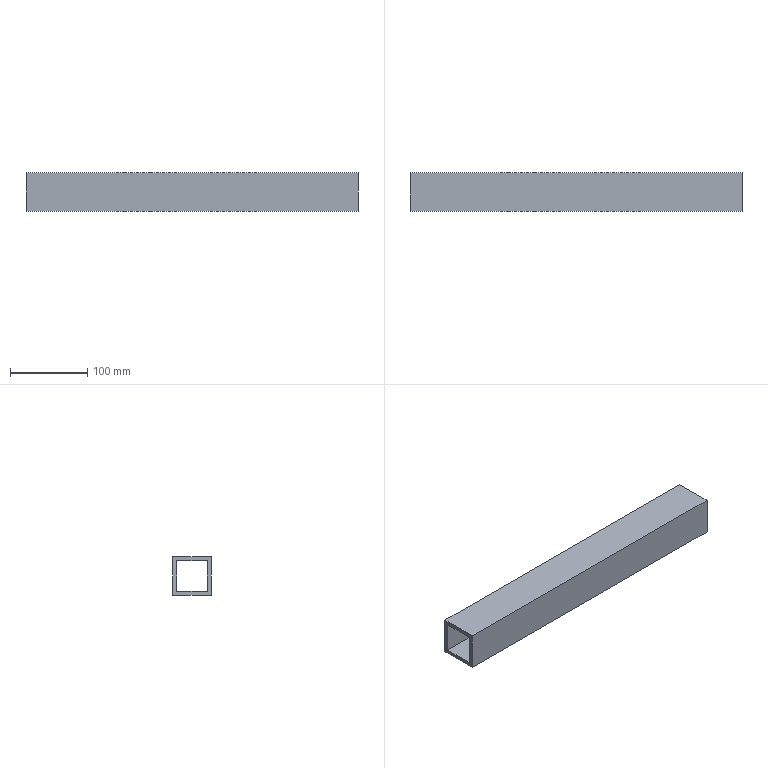Part | NX | features solid 2 | 1 solid | 10 faces | box 430 x 50 x 50 mm | volume 387000 mm3 | plane 10
STEP:
#1=CARTESIAN_POINT('',(630.,520.,-560.));
#2=VERTEX_POINT('',#1);
#3=CARTESIAN_POINT('',(630.,480.,-560.));
#4=VERTEX_POINT('',#3);
#5=CARTESIAN_POINT('',(630.,475.,-560.));
#6=DIRECTION('',(0.,-1.,0.));
#7=VECTOR('',#6,1000.);
#8=LINE('',#5,#7);
#9=EDGE_CURVE('',#2,#4,#8,.T.);
#10=ORIENTED_EDGE('',*,*,#9,.F.);
#11=CARTESIAN_POINT('',(630.,520.,-520.));
#12=VERTEX_POINT('',#11);
#13=CARTESIAN_POINT('',(630.,520.,-565.));
#14=DIRECTION('',(0.,0.,-1.));
#15=VECTOR('',#14,1000.);
#16=LINE('',#13,#15);
#17=EDGE_CURVE('',#12,#2,#16,.T.);
#18=ORIENTED_EDGE('',*,*,#17,.F.);
#19=CARTESIAN_POINT('',(630.,480.,-520.));
#20=VERTEX_POINT('',#19);
#21=CARTESIAN_POINT('',(630.,475.,-520.));
#22=DIRECTION('',(0.,1.,0.));
#23=VECTOR('',#22,1000.);
#24=LINE('',#21,#23);
#25=EDGE_CURVE('',#20,#12,#24,.T.);
#26=ORIENTED_EDGE('',*,*,#25,.F.);
#27=CARTESIAN_POINT('',(630.,480.,-565.));
#28=DIRECTION('',(0.,0.,1.));
#29=VECTOR('',#28,1000.);
#30=LINE('',#27,#29);
#31=EDGE_CURVE('',#4,#20,#30,.T.);
#32=ORIENTED_EDGE('',*,*,#31,.F.);
#33=EDGE_LOOP('',(#10,#18,#26,#32));
#34=FACE_BOUND('',#33,.T.);
#35=CARTESIAN_POINT('',(630.,475.,-515.));
#36=VERTEX_POINT('',#35);
#37=CARTESIAN_POINT('',(630.,525.,-515.));
#38=VERTEX_POINT('',#37);
#39=CARTESIAN_POINT('',(630.,475.,-515.));
#40=DIRECTION('',(0.,1.,0.));
#41=VECTOR('',#40,1000.);
#42=LINE('',#39,#41);
#43=EDGE_CURVE('',#36,#38,#42,.T.);
#44=ORIENTED_EDGE('',*,*,#43,.T.);
#45=CARTESIAN_POINT('',(630.,525.,-565.));
#46=VERTEX_POINT('',#45);
#47=CARTESIAN_POINT('',(630.,525.,-565.));
#48=DIRECTION('',(0.,0.,-1.));
#49=VECTOR('',#48,1000.);
#50=LINE('',#47,#49);
#51=EDGE_CURVE('',#38,#46,#50,.T.);
#52=ORIENTED_EDGE('',*,*,#51,.T.);
#53=CARTESIAN_POINT('',(630.,475.,-565.));
#54=VERTEX_POINT('',#53);
#55=CARTESIAN_POINT('',(630.,475.,-565.));
#56=DIRECTION('',(0.,-1.,0.));
#57=VECTOR('',#56,1000.);
#58=LINE('',#55,#57);
#59=EDGE_CURVE('',#46,#54,#58,.T.);
#60=ORIENTED_EDGE('',*,*,#59,.T.);
#61=CARTESIAN_POINT('',(630.,475.,-565.));
#62=DIRECTION('',(0.,0.,1.));
#63=VECTOR('',#62,1000.);
#64=LINE('',#61,#63);
#65=EDGE_CURVE('',#54,#36,#64,.T.);
#66=ORIENTED_EDGE('',*,*,#65,.T.);
#67=EDGE_LOOP('',(#44,#52,#60,#66));
#68=FACE_BOUND('',#67,.T.);
#69=CARTESIAN_POINT('',(630.,475.,-565.));
#70=DIRECTION('',(1.,0.,0.));
#71=DIRECTION('',(0.,-1.,0.));
#72=AXIS2_PLACEMENT_3D('',#69,#70,#71);
#73=PLANE('',#72);
#74=ADVANCED_FACE('',(#34,#68),#73,.F.);
#75=CARTESIAN_POINT('',(1060.,475.,-565.));
#76=VERTEX_POINT('',#75);
#77=CARTESIAN_POINT('',(640.,475.,-565.));
#78=DIRECTION('',(1.,0.,0.));
#79=VECTOR('',#78,1000.);
#80=LINE('',#77,#79);
#81=EDGE_CURVE('',#54,#76,#80,.T.);
#82=ORIENTED_EDGE('',*,*,#81,.T.);
#83=CARTESIAN_POINT('',(1060.,475.,-515.));
#84=VERTEX_POINT('',#83);
#85=CARTESIAN_POINT('',(1060.,475.,-565.));
#86=DIRECTION('',(0.,0.,-1.));
#87=VECTOR('',#86,1000.);
#88=LINE('',#85,#87);
#89=EDGE_CURVE('',#84,#76,#88,.T.);
#90=ORIENTED_EDGE('',*,*,#89,.F.);
#91=CARTESIAN_POINT('',(640.,475.,-515.));
#92=DIRECTION('',(-1.,0.,0.));
#93=VECTOR('',#92,1000.);
#94=LINE('',#91,#93);
#95=EDGE_CURVE('',#84,#36,#94,.T.);
#96=ORIENTED_EDGE('',*,*,#95,.T.);
#97=ORIENTED_EDGE('',*,*,#65,.F.);
#98=EDGE_LOOP('',(#82,#90,#96,#97));
#99=FACE_BOUND('',#98,.T.);
#100=CARTESIAN_POINT('',(640.,475.,-565.));
#101=DIRECTION('',(0.,1.,0.));
#102=DIRECTION('',(1.,0.,0.));
#103=AXIS2_PLACEMENT_3D('',#100,#101,#102);
#104=PLANE('',#103);
#105=ADVANCED_FACE('',(#99),#104,.F.);
#106=CARTESIAN_POINT('',(1060.,525.,-565.));
#107=VERTEX_POINT('',#106);
#108=CARTESIAN_POINT('',(640.,525.,-565.));
#109=DIRECTION('',(1.,0.,0.));
#110=VECTOR('',#109,1000.);
#111=LINE('',#108,#110);
#112=EDGE_CURVE('',#46,#107,#111,.T.);
#113=ORIENTED_EDGE('',*,*,#112,.T.);
#114=CARTESIAN_POINT('',(1060.,475.,-565.));
#115=DIRECTION('',(0.,1.,0.));
#116=VECTOR('',#115,1000.);
#117=LINE('',#114,#116);
#118=EDGE_CURVE('',#76,#107,#117,.T.);
#119=ORIENTED_EDGE('',*,*,#118,.F.);
#120=ORIENTED_EDGE('',*,*,#81,.F.);
#121=ORIENTED_EDGE('',*,*,#59,.F.);
#122=EDGE_LOOP('',(#113,#119,#120,#121));
#123=FACE_BOUND('',#122,.T.);
#124=CARTESIAN_POINT('',(640.,475.,-565.));
#125=DIRECTION('',(0.,0.,1.));
#126=DIRECTION('',(0.,-1.,0.));
#127=AXIS2_PLACEMENT_3D('',#124,#125,#126);
#128=PLANE('',#127);
#129=ADVANCED_FACE('',(#123),#128,.F.);
#130=CARTESIAN_POINT('',(1060.,525.,-515.));
#131=VERTEX_POINT('',#130);
#132=CARTESIAN_POINT('',(640.,525.,-515.));
#133=DIRECTION('',(1.,0.,0.));
#134=VECTOR('',#133,1000.);
#135=LINE('',#132,#134);
#136=EDGE_CURVE('',#38,#131,#135,.T.);
#137=ORIENTED_EDGE('',*,*,#136,.T.);
#138=CARTESIAN_POINT('',(1060.,525.,-515.));
#139=DIRECTION('',(0.,0.,1.));
#140=VECTOR('',#139,1000.);
#141=LINE('',#138,#140);
#142=EDGE_CURVE('',#107,#131,#141,.T.);
#143=ORIENTED_EDGE('',*,*,#142,.F.);
#144=ORIENTED_EDGE('',*,*,#112,.F.);
#145=ORIENTED_EDGE('',*,*,#51,.F.);
#146=EDGE_LOOP('',(#137,#143,#144,#145));
#147=FACE_BOUND('',#146,.T.);
#148=CARTESIAN_POINT('',(640.,525.,-515.));
#149=DIRECTION('',(0.,-1.,0.));
#150=DIRECTION('',(-1.,0.,0.));
#151=AXIS2_PLACEMENT_3D('',#148,#149,#150);
#152=PLANE('',#151);
#153=ADVANCED_FACE('',(#147),#152,.F.);
#154=ORIENTED_EDGE('',*,*,#95,.F.);
#155=CARTESIAN_POINT('',(1060.,475.,-515.));
#156=DIRECTION('',(0.,-1.,0.));
#157=VECTOR('',#156,1000.);
#158=LINE('',#155,#157);
#159=EDGE_CURVE('',#131,#84,#158,.T.);
#160=ORIENTED_EDGE('',*,*,#159,.F.);
#161=ORIENTED_EDGE('',*,*,#136,.F.);
#162=ORIENTED_EDGE('',*,*,#43,.F.);
#163=EDGE_LOOP('',(#154,#160,#161,#162));
#164=FACE_BOUND('',#163,.T.);
#165=CARTESIAN_POINT('',(1060.,475.,-515.));
#166=DIRECTION('',(0.,0.,-1.));
#167=DIRECTION('',(-1.,0.,0.));
#168=AXIS2_PLACEMENT_3D('',#165,#166,#167);
#169=PLANE('',#168);
#170=ADVANCED_FACE('',(#164),#169,.F.);
#171=CARTESIAN_POINT('',(1060.,520.,-560.));
#172=VERTEX_POINT('',#171);
#173=CARTESIAN_POINT('',(1060.,480.,-560.));
#174=VERTEX_POINT('',#173);
#175=CARTESIAN_POINT('',(1060.,475.,-560.));
#176=DIRECTION('',(0.,-1.,0.));
#177=VECTOR('',#176,1000.);
#178=LINE('',#175,#177);
#179=EDGE_CURVE('',#172,#174,#178,.T.);
#180=ORIENTED_EDGE('',*,*,#179,.F.);
#181=CARTESIAN_POINT('',(640.,520.,-560.));
#182=DIRECTION('',(1.,0.,0.));
#183=VECTOR('',#182,1000.);
#184=LINE('',#181,#183);
#185=EDGE_CURVE('',#2,#172,#184,.T.);
#186=ORIENTED_EDGE('',*,*,#185,.F.);
#187=ORIENTED_EDGE('',*,*,#9,.T.);
#188=CARTESIAN_POINT('',(640.,480.,-560.));
#189=DIRECTION('',(-1.,0.,0.));
#190=VECTOR('',#189,1000.);
#191=LINE('',#188,#190);
#192=EDGE_CURVE('',#174,#4,#191,.T.);
#193=ORIENTED_EDGE('',*,*,#192,.F.);
#194=EDGE_LOOP('',(#180,#186,#187,#193));
#195=FACE_BOUND('',#194,.T.);
#196=CARTESIAN_POINT('',(640.,520.,-560.));
#197=DIRECTION('',(0.,0.,1.));
#198=DIRECTION('',(0.,-1.,0.));
#199=AXIS2_PLACEMENT_3D('',#196,#197,#198);
#200=PLANE('',#199);
#201=ADVANCED_FACE('',(#195),#200,.T.);
#202=CARTESIAN_POINT('',(1060.,480.,-520.));
#203=VERTEX_POINT('',#202);
#204=CARTESIAN_POINT('',(1060.,480.,-565.));
#205=DIRECTION('',(0.,0.,1.));
#206=VECTOR('',#205,1000.);
#207=LINE('',#204,#206);
#208=EDGE_CURVE('',#174,#203,#207,.T.);
#209=ORIENTED_EDGE('',*,*,#208,.F.);
#210=ORIENTED_EDGE('',*,*,#192,.T.);
#211=ORIENTED_EDGE('',*,*,#31,.T.);
#212=CARTESIAN_POINT('',(1060.,480.,-520.));
#213=DIRECTION('',(-1.,0.,0.));
#214=VECTOR('',#213,1000.);
#215=LINE('',#212,#214);
#216=EDGE_CURVE('',#203,#20,#215,.T.);
#217=ORIENTED_EDGE('',*,*,#216,.F.);
#218=EDGE_LOOP('',(#209,#210,#211,#217));
#219=FACE_BOUND('',#218,.T.);
#220=CARTESIAN_POINT('',(1060.,480.,-560.));
#221=DIRECTION('',(0.,1.,0.));
#222=DIRECTION('',(1.,0.,0.));
#223=AXIS2_PLACEMENT_3D('',#220,#221,#222);
#224=PLANE('',#223);
#225=ADVANCED_FACE('',(#219),#224,.T.);
#226=CARTESIAN_POINT('',(1060.,520.,-520.));
#227=VERTEX_POINT('',#226);
#228=CARTESIAN_POINT('',(1060.,475.,-520.));
#229=DIRECTION('',(0.,1.,0.));
#230=VECTOR('',#229,1000.);
#231=LINE('',#228,#230);
#232=EDGE_CURVE('',#203,#227,#231,.T.);
#233=ORIENTED_EDGE('',*,*,#232,.F.);
#234=ORIENTED_EDGE('',*,*,#216,.T.);
#235=ORIENTED_EDGE('',*,*,#25,.T.);
#236=CARTESIAN_POINT('',(1060.,520.,-520.));
#237=DIRECTION('',(-1.,0.,0.));
#238=VECTOR('',#237,1000.);
#239=LINE('',#236,#238);
#240=EDGE_CURVE('',#227,#12,#239,.T.);
#241=ORIENTED_EDGE('',*,*,#240,.F.);
#242=EDGE_LOOP('',(#233,#234,#235,#241));
#243=FACE_BOUND('',#242,.T.);
#244=CARTESIAN_POINT('',(1060.,480.,-520.));
#245=DIRECTION('',(0.,0.,-1.));
#246=DIRECTION('',(-1.,0.,0.));
#247=AXIS2_PLACEMENT_3D('',#244,#245,#246);
#248=PLANE('',#247);
#249=ADVANCED_FACE('',(#243),#248,.T.);
#250=CARTESIAN_POINT('',(1060.,520.,-565.));
#251=DIRECTION('',(0.,0.,-1.));
#252=VECTOR('',#251,1000.);
#253=LINE('',#250,#252);
#254=EDGE_CURVE('',#227,#172,#253,.T.);
#255=ORIENTED_EDGE('',*,*,#254,.F.);
#256=ORIENTED_EDGE('',*,*,#240,.T.);
#257=ORIENTED_EDGE('',*,*,#17,.T.);
#258=ORIENTED_EDGE('',*,*,#185,.T.);
#259=EDGE_LOOP('',(#255,#256,#257,#258));
#260=FACE_BOUND('',#259,.T.);
#261=CARTESIAN_POINT('',(640.,520.,-520.));
#262=DIRECTION('',(0.,-1.,0.));
#263=DIRECTION('',(-1.,0.,0.));
#264=AXIS2_PLACEMENT_3D('',#261,#262,#263);
#265=PLANE('',#264);
#266=ADVANCED_FACE('',(#260),#265,.T.);
#267=ORIENTED_EDGE('',*,*,#232,.T.);
#268=ORIENTED_EDGE('',*,*,#254,.T.);
#269=ORIENTED_EDGE('',*,*,#179,.T.);
#270=ORIENTED_EDGE('',*,*,#208,.T.);
#271=EDGE_LOOP('',(#267,#268,#269,#270));
#272=FACE_BOUND('',#271,.T.);
#273=ORIENTED_EDGE('',*,*,#142,.T.);
#274=ORIENTED_EDGE('',*,*,#159,.T.);
#275=ORIENTED_EDGE('',*,*,#89,.T.);
#276=ORIENTED_EDGE('',*,*,#118,.T.);
#277=EDGE_LOOP('',(#273,#274,#275,#276));
#278=FACE_BOUND('',#277,.T.);
#279=CARTESIAN_POINT('',(1060.,475.,-565.));
#280=DIRECTION('',(1.,0.,0.));
#281=DIRECTION('',(0.,-1.,0.));
#282=AXIS2_PLACEMENT_3D('',#279,#280,#281);
#283=PLANE('',#282);
#284=ADVANCED_FACE('',(#272,#278),#283,.T.);
#285=CLOSED_SHELL('',(#74,#105,#129,#153,#170,#201,#225,#249,#266,#284));
#286=MANIFOLD_SOLID_BREP('',#285);
#287=(LENGTH_UNIT()NAMED_UNIT(*)SI_UNIT(.MILLI.,.METRE.));
#288=UNCERTAINTY_MEASURE_WITH_UNIT(LENGTH_MEASURE(0.00001),#287,'','');
#289=(NAMED_UNIT(*)PLANE_ANGLE_UNIT()SI_UNIT($,.RADIAN.));
#290=(NAMED_UNIT(*)SI_UNIT($,.STERADIAN.)SOLID_ANGLE_UNIT());
#291=(GEOMETRIC_REPRESENTATION_CONTEXT(3)GLOBAL_UNCERTAINTY_ASSIGNED_CONTEXT((#288))GLOBAL_UNIT_ASSIGNED_CONTEXT((#287,#289,#290))REPRESENTATION_CONTEXT('',''));
#292=ADVANCED_BREP_SHAPE_REPRESENTATION('',(#286),#291);